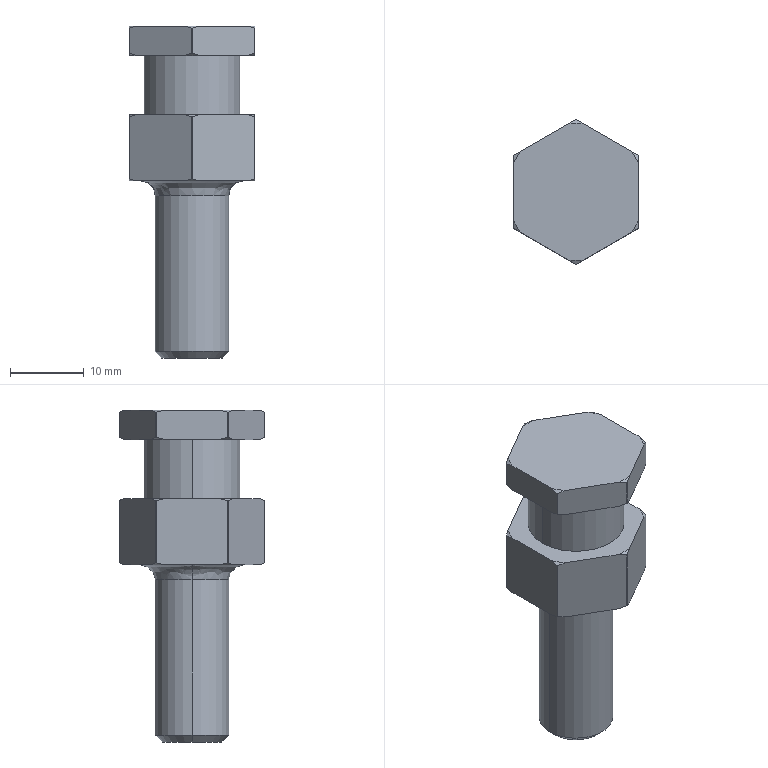Part | SolidWorks | features BaseBody 1 | 1 solid | 62 faces | box 17 x 19.6 x 45 mm | volume 6217 mm3 | cone 27 | plane 17 | cylinder 16 | spline 2 | commonest cylinder face diameters 19.6 x12 10 x2 13 x2